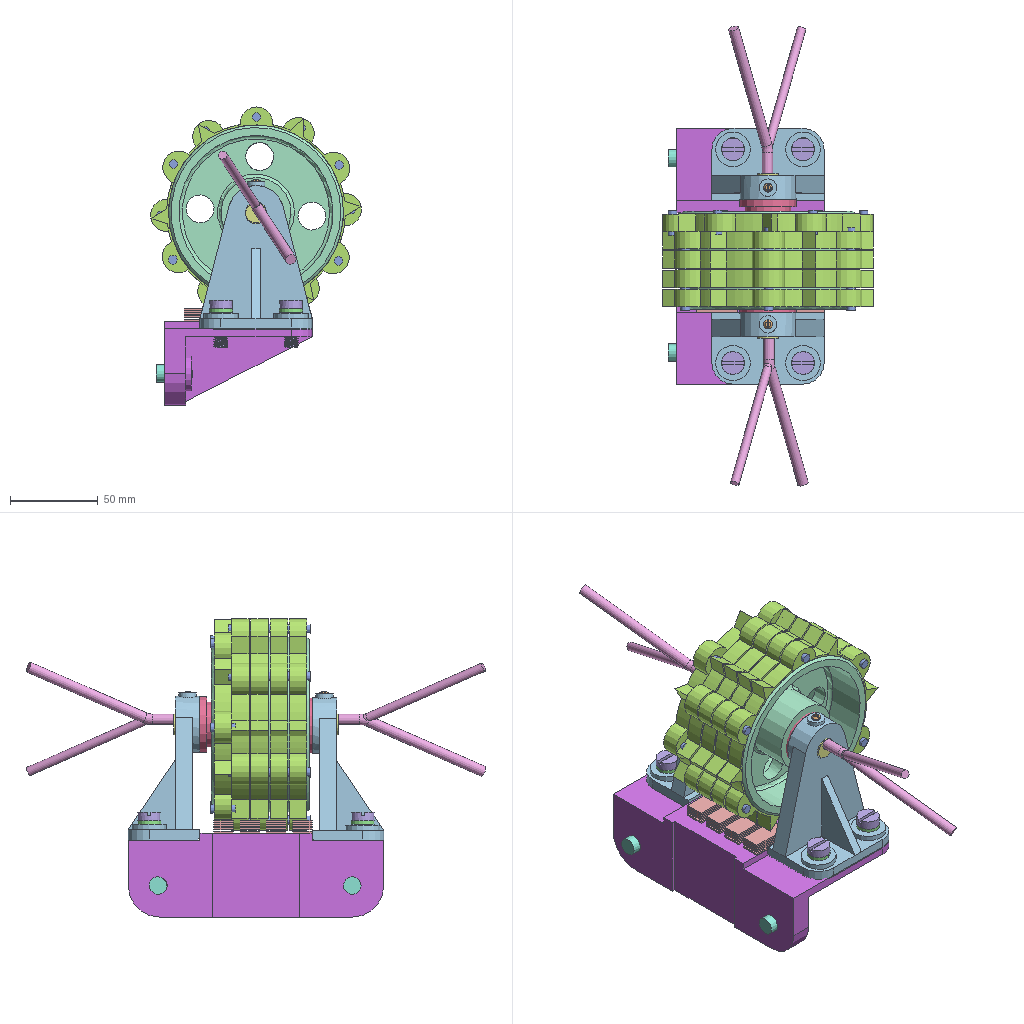Assembly | NX | 13 different items | 119 placed | box 121 x 263 x 170 mm
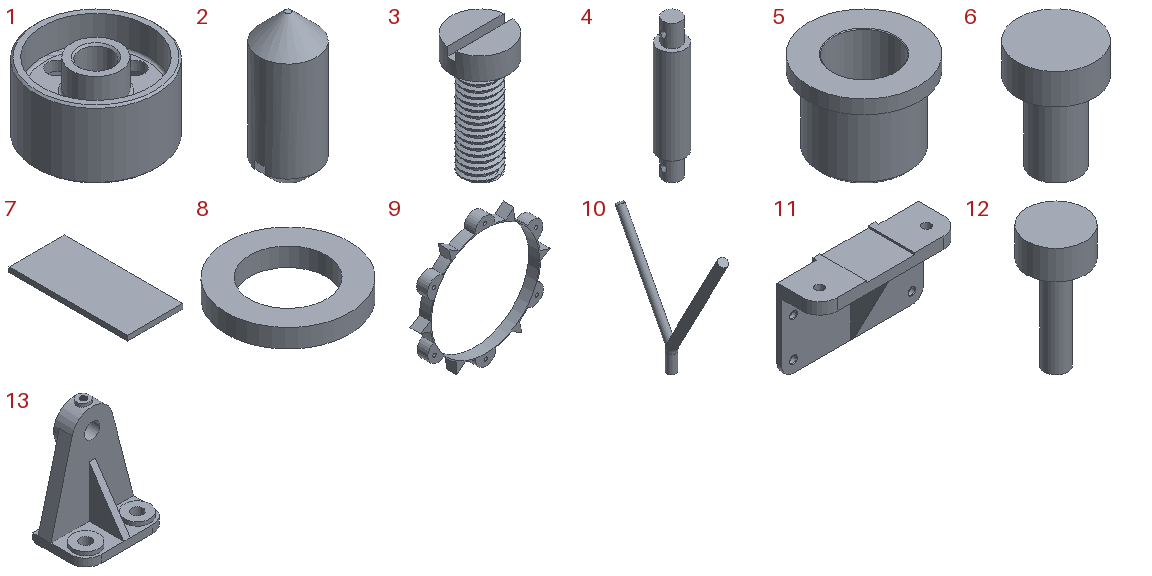Parts list (item | quantity | size | volume | features):
1 | x1 | 100 x 100 x 56 mm | 171833 mm3 | features EXTRUDE 5, DATUM_CSYS 3, CHAMFER 2, SKETCH 2, BLEND 1
2 | x2 | 5 x 5 x 12 mm | 194.481 mm3 | features CHAMFER 2, DATUM_CSYS 2, CYLINDER 1, EXTRUDE 1, SKETCH 1
3 | x4 | 13 x 13 x 27 mm | 1535 mm3 | features CYLINDER 3, DATUM_CSYS 2, TRIM BODY 2, DATUM_PLANE 1, EXTRUDE 1, SKETCH 1, THREADS 1
4 | x1 | 18 x 18 x 94 mm | 19453 mm3 | features CYLINDER 3, DATUM_CSYS 3, SUBTRACT 3, SKETCH 2, SWP104 2, CHAMFER 1, DATUM_PLANE 1, EXTRUDE 1, SPHERE 1
5 | x2 | 32 x 32 x 24 mm | 7686 mm3 | features CHAMFER 2, DATUM_CSYS 2, EXTRUDE 2, SKETCH 1
6 | x65 | 5 x 5 x 7 mm | 74.613 mm3 | features CYLINDER 2, DATUM_CSYS 1
7 | x28 | 11.058 x 23.696 x 1 mm | 262.025 mm3 | features DATUM_CSYS 2, EXTRUDE 1, SKETCH 1
8 | x4 | 13.2 x 13.2 x 2 mm | 168.075 mm3 | features CYLINDER 2, DATUM_CSYS 1
9 | x5 | 119.85 x 10 x 120.564 mm | 13504 mm3 | features DATUM_CSYS 3, EXTRUDE 2, SKETCH 2
10 | x2 | 6 x 76.071 x 84.286 mm | 4037 mm3 | features DATUM_CSYS 2, SWP104 2, SKETCH 1
11 | x1 | 146 x 48 x 84 mm | 149346 mm3 | features DATUM_CSYS 6, SIMPLE HOLE 6, SKETCH 5, SYMBOLIC_THREAD 4, EXTRUDE 3, CYLINDER 2, HOLE PACKAGE 2, BLEND 1, CPROJ 1, Intersection Curve 1, RIB 1
12 | x2 | 10 x 10 x 21 mm | 593.761 mm3 | features CYLINDER 2, DATUM_CSYS 1
13 | x2 | 64 x 41 x 84 mm | 53505 mm3 | features EXTRUDE 7, DATUM_CSYS 6, SKETCH 5, CHAMFER 1, CPROJ 1, CYLINDER 1, Intersection Curve 1, RIB 1, SUBTRACT 1, THREADS 1
Mates (type | each side: item.copy, entity, surface, feature):
Fix | 11.1 component | 2 times
Concentric | 13.1 edge | 11.1 edge | 2 times
Fix | 13.1 component
Concentric | 5.1 edge | 13.1 edge | 2 times
Concentric | 4.1 edge | 13.1 edge
Touch | 1.1 face cylinder Extrude(5) | 4.1 face cylinder Cylinder(2)
Concentric | 8.1 edge | 13.1 edge
Concentric | 3.1 edge | 8.1 edge
Fix | assembly component | 4 times
Bond | 8.1 component | assembly component | 6 times
Bond | 3.1 component | assembly component | 6 times
LinearPattern | assembly axis | assembly csys | assembly csys | 7 times
Concentric | 2.1 edge | 13.1 edge
Bond | 2.1 component | assembly component | 2 times
Parallel | 2.1 face plane Extrude(5) | 13.1 face cylinder Extrude(5)
Concentric | 12.1 edge | 11.1 edge
Concentric | 9.1 edge | 1.1 edge | 2 times
Distance | 10.1 face cylinder Tube(4) | 4.1 face cylinder Cylinder(3)
Distance | 10.1 face cylinder Tube(4) | 4.1 face cylinder Cylinder(1)
Concentric | 6.1 edge | 9.1 edge | 4 times
Touch | 7.1 face plane Extrude(1) | 13.1 face plane Extrude(2)
Touch | 7.1 face plane Extrude(1) | 11.1 face plane Extrude(4) | 2 times